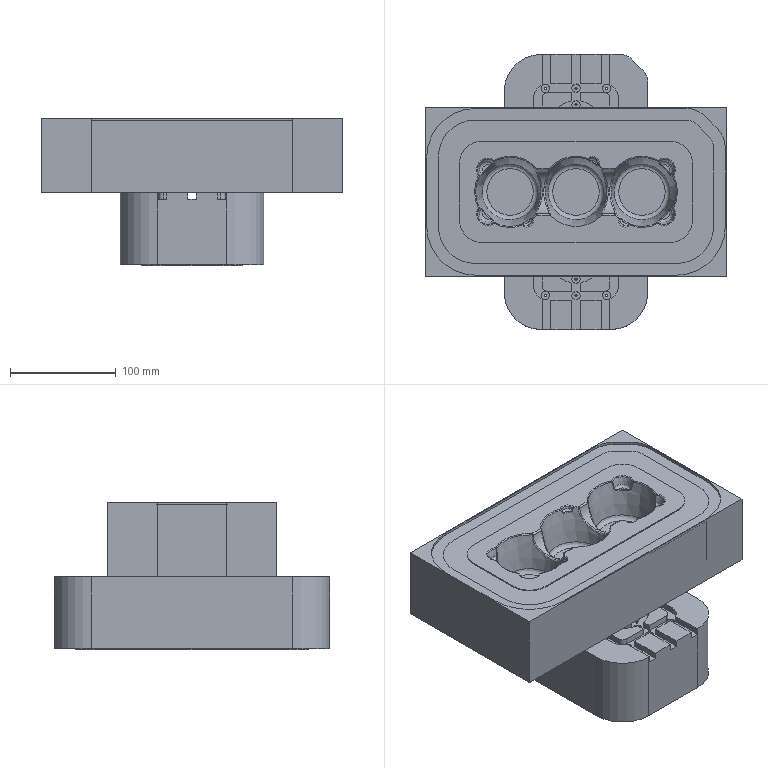NC program | NX | posted with a generic post | part box 284.317 x 260.317 x 139.5 mm
Lines 198484 to 199234 of 226982:
(B6 , TOOL : D10)
N396948 M6
N396950 G53
N396952 G17 G0 G90 X62.725 Y73.878 S7000 M3 M8
N396954 G43 Z220.5 H0
N396956 Z70.
N396958 G94 G1 X100.887 Z68. F4000.
N396960 X103.946
N396962 G2 X118.795 Y67.727 R21.
N396964 G1 X130.008 Y56.514
N396966 G2 X136.159 Y41.664 R21.
N396968 G1 Y-32.878
N396970 G2 X95.159 Y-73.878 R41.
N396972 G1 X-95.159
N396974 G2 X-136.159 Y-32.878 R41.
N396976 G1 Y32.878
N396978 G2 X-95.159 Y73.878 R41.
N396980 G1 X100.887
N396982 Y66.878
N396984 X103.946
N396986 G2 X113.845 Y62.777 R14.
N396988 G1 X125.058 Y51.564
N396990 G2 X129.159 Y41.664 R14.
N396992 G1 Y-32.878
N396994 G2 X95.159 Y-66.878 R34.
N396996 G1 X-95.159
N396998 G2 X-129.159 Y-32.878 R34.
N397000 G1 Y32.878
N397002 G2 X-95.159 Y66.878 R34.
N397004 G1 X100.887
N397006 Y59.878
N397008 X103.946
N397010 G2 X108.895 Y57.827 R7.
N397012 G1 X120.108 Y46.614
N397014 G2 X122.159 Y41.664 R7.
N397016 G1 Y-32.878
N397018 G2 X100.008 Y-59.439 R27.
N397020 G1 X98.751 Y-52.552
N397022 G3 X114.834 Y-36.469 R27.372
N397024 G2 X98.751 Y-52.552 R20.
N397026 G1 X93.926 Y-53.864
N397028 G2 X89.187 Y-54.278 R27.372
N397030 G1 X-89.187
N397032 G2 X-93.926 Y-53.864 R27.372
N397034 X-94.324 Y-54.878 R5.
N397036 G1 X94.324
N397038 G2 X93.926 Y-53.864 R5.
N397040 G1 X98.751 Y-52.552
N397042 X100.008 Y-59.439
N397044 G2 X95.159 Y-59.878 R27.
N397046 G1 X-95.159
N397048 G2 X-121.72 Y-37.726 R27.
N397050 G1 X-114.834 Y-36.469
N397052 G3 X-98.751 Y-52.552 R27.372
N397054 G2 X-114.834 Y-36.469 R20.
N397056 G1 X-121.72 Y-37.726
N397058 G2 X-122.159 Y-32.878 R27.
N397060 G1 Y32.878
N397062 G2 X-100.008 Y59.439 R27.
N397064 G1 X-98.751 Y52.552
N397066 G3 X-114.834 Y36.469 R27.372
N397068 G1 X-117.159 Y32.043
N397070 Y-32.043
N397072 G2 X-116.145 Y-31.644 R5.
N397074 X-116.559 Y-26.906 R27.372
N397076 G1 Y26.906
N397078 G2 X-116.145 Y31.644 R27.372
N397080 X-117.159 Y32.043 R5.
N397082 G1 X-114.834 Y36.469
N397084 G2 X-98.751 Y52.552 R20.
N397086 G1 X-93.926 Y53.864
N397088 G2 X-89.187 Y54.278 R27.372
N397090 G1 X89.187
N397092 G2 X92.96 Y54.016 R27.372
N397094 X93.246 Y54.878 R5.
N397096 G1 X-94.324
N397098 G2 X-93.926 Y53.864 R5.
N397100 G1 X-98.751 Y52.552
N397102 X-100.008 Y59.439
N397104 G2 X-95.159 Y59.878 R27.
N397106 G1 X100.887
N397108 Y52.878
N397110 X103.946
N397112 X115.159 Y41.664
N397114 Y35.547
N397116 X116.297 Y30.679
N397118 G2 X116.559 Y26.906 R27.372
N397120 G1 Y-26.906
N397122 G2 X116.145 Y-31.644 R27.372
N397124 X117.159 Y-32.043 R5.
N397126 G1 Y30.965
N397128 G2 X116.297 Y30.679 R5.
N397130 G1 X115.159 Y35.547
N397132 G3 X97.829 Y52.878 R27.372
N397134 G1 X97.387 Y51.549
N397136 G2 X115.159 Y26.906 R25.972
N397138 G1 Y-26.906
N397140 G2 X89.187 Y-52.878 R25.972
N397142 G1 X-89.187
N397144 G2 X-115.159 Y-26.906 R25.972
N397146 G1 Y26.906
N397148 G2 X-89.187 Y52.878 R25.972
N397150 G1 X89.187
N397152 G2 X97.387 Y51.549 R25.972
N397154 G1 X97.829 Y52.878
N397156 X100.887
N397158 G3 X102.887 Y54.878 R2.
N397160 G1 Z69.
N397162 G0 Z220.5
(B7 , TOOL : D10)
N397164 X53.127 Y72.878
N397166 Z69.
N397168 G1 X105.041 Z68.955
N397170 X107.727 Y72.547 Z68.952
N397172 X110.343 Y71.858 Z68.95
N397174 X112.843 Y70.823 Z68.948
N397176 X115.18 Y69.46 Z68.945
N397178 X117.313 Y67.795 Z68.943
N397180 X130.076 Y55.032 Z68.927
N397182 X131.741 Y52.899 Z68.925
N397184 X133.104 Y50.562 Z68.922
N397186 X134.14 Y48.062 Z68.92
N397188 X134.829 Y45.446 Z68.918
N397190 X135.159 Y42.76 Z68.915
N397192 Y-34.427 Z68.848
N397194 X134.766 Y-38.677 Z68.844
N397196 X133.924 Y-42.861 Z68.841
N397198 X132.641 Y-46.931 Z68.837
N397200 X130.931 Y-50.842 Z68.833
N397202 X128.815 Y-54.548 Z68.829
N397204 X126.317 Y-58.009 Z68.826
N397206 X123.464 Y-61.183 Z68.822
N397208 X120.29 Y-64.036 Z68.818
N397210 X116.83 Y-66.534 Z68.814
N397212 X113.123 Y-68.65 Z68.811
N397214 X109.212 Y-70.359 Z68.807
N397216 X105.142 Y-71.643 Z68.803
N397218 X100.958 Y-72.485 Z68.8
N397220 X96.708 Y-72.878 Z68.796
N397222 X-96.708 Z68.627
N397224 X-100.958 Y-72.485 Z68.623
N397226 X-105.142 Y-71.643 Z68.62
N397228 X-109.212 Y-70.359 Z68.616
N397230 X-113.123 Y-68.65 Z68.612
N397232 X-116.83 Y-66.534 Z68.608
N397234 X-120.29 Y-64.036 Z68.605
N397236 X-123.464 Y-61.183 Z68.601
N397238 X-126.317 Y-58.009 Z68.597
N397240 X-128.815 Y-54.548 Z68.594
N397242 X-130.931 Y-50.842 Z68.59
N397244 X-132.641 Y-46.931 Z68.586
N397246 X-133.924 Y-42.861 Z68.582
N397248 X-134.766 Y-38.677 Z68.579
N397250 X-135.159 Y-34.427 Z68.575
N397252 Y34.427 Z68.515
N397254 X-134.766 Y38.677 Z68.511
N397256 X-133.924 Y42.861 Z68.507
N397258 X-132.641 Y46.931 Z68.504
N397260 X-130.931 Y50.842 Z68.5
N397262 X-128.815 Y54.548 Z68.496
N397264 X-126.317 Y58.009 Z68.492
N397266 X-123.464 Y61.183 Z68.489
N397268 X-120.29 Y64.036 Z68.485
N397270 X-116.83 Y66.534 Z68.481
N397272 X-113.123 Y68.65 Z68.478
N397274 X-109.212 Y70.359 Z68.474
N397276 X-105.142 Y71.643 Z68.47
N397278 X-100.958 Y72.485 Z68.466
N397280 X-96.708 Y72.878 Z68.463
N397282 X105.041 Z68.287
N397284 X107.727 Y72.547 Z68.284
N397286 X110.343 Y71.858 Z68.282
N397288 X112.843 Y70.823 Z68.28
N397290 X115.18 Y69.46 Z68.277
N397292 X117.313 Y67.795 Z68.275
N397294 X130.076 Y55.032 Z68.259
N397296 X131.741 Y52.899 Z68.257
N397298 X133.104 Y50.562 Z68.254
N397300 X134.14 Y48.062 Z68.252
N397302 X134.829 Y45.446 Z68.25
N397304 X135.159 Y42.76 Z68.247
N397306 Y-34.427 Z68.18
N397308 X134.766 Y-38.677 Z68.176
N397310 X133.924 Y-42.861 Z68.172
N397312 X132.641 Y-46.931 Z68.169
N397314 X130.931 Y-50.842 Z68.165
N397316 X128.815 Y-54.548 Z68.161
N397318 X126.317 Y-58.009 Z68.158
N397320 X123.464 Y-61.183 Z68.154
N397322 X120.29 Y-64.036 Z68.15
N397324 X116.83 Y-66.534 Z68.146
N397326 X113.123 Y-68.65 Z68.143
N397328 X109.212 Y-70.359 Z68.139
N397330 X105.142 Y-71.643 Z68.135
N397332 X100.958 Y-72.485 Z68.131
N397334 X96.708 Y-72.878 Z68.128
N397336 X-96.708 Z67.959
N397338 X-100.958 Y-72.485 Z67.955
N397340 X-105.142 Y-71.643 Z67.952
N397342 X-109.212 Y-70.359 Z67.948
N397344 X-113.123 Y-68.65 Z67.944
N397346 X-116.83 Y-66.534 Z67.94
N397348 X-120.29 Y-64.036 Z67.937
N397350 X-123.464 Y-61.183 Z67.933
N397352 X-126.317 Y-58.009 Z67.929
N397354 X-128.815 Y-54.548 Z67.925
N397356 X-130.931 Y-50.842 Z67.922
N397358 X-132.641 Y-46.931 Z67.918
N397360 X-133.924 Y-42.861 Z67.914
N397362 X-134.766 Y-38.677 Z67.911
N397364 X-135.159 Y-34.427 Z67.907
N397366 Y34.427 Z67.847
N397368 X-134.766 Y38.677 Z67.843
N397370 X-133.924 Y42.861 Z67.839
N397372 X-132.641 Y46.931 Z67.836
N397374 X-130.931 Y50.842 Z67.832
N397376 X-128.815 Y54.548 Z67.828
N397378 X-126.317 Y58.009 Z67.824
N397380 X-123.464 Y61.183 Z67.821
N397382 X-120.29 Y64.036 Z67.817
N397384 X-116.83 Y66.534 Z67.813
N397386 X-113.123 Y68.65 Z67.809
N397388 X-109.212 Y70.359 Z67.806
N397390 X-105.142 Y71.643 Z67.802
N397392 X-100.958 Y72.485 Z67.798
N397394 X-96.708 Y72.878 Z67.795
N397396 X105.041 Z67.619
N397398 X107.727 Y72.547 Z67.616
N397400 X110.343 Y71.858 Z67.614
N397402 X112.843 Y70.823 Z67.611
N397404 X115.18 Y69.46 Z67.609
N397406 X117.313 Y67.795 Z67.607
N397408 X130.076 Y55.032 Z67.591
N397410 X131.741 Y52.899 Z67.589
N397412 X133.104 Y50.562 Z67.586
N397414 X134.14 Y48.062 Z67.584
N397416 X134.829 Y45.446 Z67.582
N397418 X135.159 Y42.76 Z67.579
N397420 Y-34.427 Z67.512
N397422 X134.766 Y-38.677 Z67.508
N397424 X133.924 Y-42.861 Z67.504
N397426 X132.641 Y-46.931 Z67.501
N397428 X130.931 Y-50.842 Z67.497
N397430 X128.815 Y-54.548 Z67.493
N397432 X126.317 Y-58.009 Z67.489
N397434 X123.464 Y-61.183 Z67.486
N397436 X120.29 Y-64.036 Z67.482
N397438 X116.83 Y-66.534 Z67.478
N397440 X113.123 Y-68.65 Z67.475
N397442 X109.212 Y-70.359 Z67.471
N397444 X105.142 Y-71.643 Z67.467
N397446 X100.958 Y-72.485 Z67.463
N397448 X96.708 Y-72.878 Z67.46
N397450 X-96.708 Z67.291
N397452 X-100.958 Y-72.485 Z67.287
N397454 X-105.142 Y-71.643 Z67.283
N397456 X-109.212 Y-70.359 Z67.28
N397458 X-113.123 Y-68.65 Z67.276
N397460 X-116.83 Y-66.534 Z67.272
N397462 X-120.29 Y-64.036 Z67.269
N397464 X-123.464 Y-61.183 Z67.265
N397466 X-126.317 Y-58.009 Z67.261
N397468 X-128.815 Y-54.548 Z67.257
N397470 X-130.931 Y-50.842 Z67.254
N397472 X-132.641 Y-46.931 Z67.25
N397474 X-133.924 Y-42.861 Z67.246
N397476 X-134.766 Y-38.677 Z67.242
N397478 X-135.159 Y-34.427 Z67.239
N397480 Y34.427 Z67.179
N397482 X-134.766 Y38.677 Z67.175
N397484 X-133.924 Y42.861 Z67.171
N397486 X-132.641 Y46.931 Z67.167
N397488 X-130.931 Y50.842 Z67.164
N397490 X-128.815 Y54.548 Z67.16
N397492 X-126.317 Y58.009 Z67.156
N397494 X-123.464 Y61.183 Z67.153
N397496 X-120.29 Y64.036 Z67.149
N397498 X-116.83 Y66.534 Z67.145
N397500 X-113.123 Y68.65 Z67.141
N397502 X-109.212 Y70.359 Z67.138
N397504 X-105.142 Y71.643 Z67.134
N397506 X-100.958 Y72.485 Z67.13
N397508 X-96.708 Y72.878 Z67.127
N397510 X105.041 Z66.95
N397512 X107.727 Y72.547 Z66.948
N397514 X110.343 Y71.858 Z66.946
N397516 X112.843 Y70.823 Z66.943
N397518 X115.18 Y69.46 Z66.941
N397520 X117.313 Y67.795 Z66.939
N397522 X130.076 Y55.032 Z66.923
N397524 X131.741 Y52.899 Z66.921
N397526 X133.104 Y50.562 Z66.918
N397528 X134.14 Y48.062 Z66.916
N397530 X134.829 Y45.446 Z66.913
N397532 X135.159 Y42.76 Z66.911
N397534 Y-34.427 Z66.844
N397536 X134.766 Y-38.677 Z66.84
N397538 X133.924 Y-42.861 Z66.836
N397540 X132.641 Y-46.931 Z66.833
N397542 X130.931 Y-50.842 Z66.829
N397544 X128.815 Y-54.548 Z66.825
N397546 X126.317 Y-58.009 Z66.821
N397548 X123.464 Y-61.183 Z66.818
N397550 X120.29 Y-64.036 Z66.814
N397552 X116.83 Y-66.534 Z66.81
N397554 X113.123 Y-68.65 Z66.806
N397556 X109.212 Y-70.359 Z66.803
N397558 X105.142 Y-71.643 Z66.799
N397560 X100.958 Y-72.485 Z66.795
N397562 X96.708 Y-72.878 Z66.792
N397564 X-96.708 Z66.623
N397566 X-100.958 Y-72.485 Z66.619
N397568 X-105.142 Y-71.643 Z66.615
N397570 X-109.212 Y-70.359 Z66.612
N397572 X-113.123 Y-68.65 Z66.608
N397574 X-116.83 Y-66.534 Z66.604
N397576 X-120.29 Y-64.036 Z66.6
N397578 X-123.464 Y-61.183 Z66.597
N397580 X-126.317 Y-58.009 Z66.593
N397582 X-128.815 Y-54.548 Z66.589
N397584 X-130.931 Y-50.842 Z66.586
N397586 X-132.641 Y-46.931 Z66.582
N397588 X-133.924 Y-42.861 Z66.578
N397590 X-134.766 Y-38.677 Z66.574
N397592 X-135.159 Y-34.427 Z66.571
N397594 Y34.427 Z66.511
N397596 X-134.766 Y38.677 Z66.507
N397598 X-133.924 Y42.861 Z66.503
N397600 X-132.641 Y46.931 Z66.499
N397602 X-130.931 Y50.842 Z66.496
N397604 X-128.815 Y54.548 Z66.492
N397606 X-126.317 Y58.009 Z66.488
N397608 X-123.464 Y61.183 Z66.484
N397610 X-120.29 Y64.036 Z66.481
N397612 X-116.83 Y66.534 Z66.477
N397614 X-113.123 Y68.65 Z66.473
N397616 X-109.212 Y70.359 Z66.47
N397618 X-105.142 Y71.643 Z66.466
N397620 X-100.958 Y72.485 Z66.462
N397622 X-96.708 Y72.878 Z66.458
N397624 X105.041 Z66.282
N397626 X107.727 Y72.547 Z66.28
N397628 X110.343 Y71.858 Z66.278
N397630 X112.843 Y70.823 Z66.275
N397632 X115.18 Y69.46 Z66.273
N397634 X117.313 Y67.795 Z66.271
N397636 X130.076 Y55.032 Z66.255
N397638 X131.741 Y52.899 Z66.252
N397640 X133.104 Y50.562 Z66.25
N397642 X134.14 Y48.062 Z66.248
N397644 X134.829 Y45.446 Z66.245
N397646 X135.159 Y42.76 Z66.243
N397648 Y-34.427 Z66.176
N397650 X134.766 Y-38.677 Z66.172
N397652 X133.924 Y-42.861 Z66.168
N397654 X132.641 Y-46.931 Z66.164
N397656 X130.931 Y-50.842 Z66.161
N397658 X128.815 Y-54.548 Z66.157
N397660 X126.317 Y-58.009 Z66.153
N397662 X123.464 Y-61.183 Z66.15
N397664 X120.29 Y-64.036 Z66.146
N397666 X116.83 Y-66.534 Z66.142
N397668 X113.123 Y-68.65 Z66.138
N397670 X109.212 Y-70.359 Z66.135
N397672 X105.142 Y-71.643 Z66.131
N397674 X100.958 Y-72.485 Z66.127
N397676 X96.708 Y-72.878 Z66.124
N397678 X-96.708 Z65.955
N397680 X-100.958 Y-72.485 Z65.951
N397682 X-105.142 Y-71.643 Z65.947
N397684 X-109.212 Y-70.359 Z65.944
N397686 X-113.123 Y-68.65 Z65.94
N397688 X-116.83 Y-66.534 Z65.936
N397690 X-120.29 Y-64.036 Z65.932
N397692 X-123.464 Y-61.183 Z65.929
N397694 X-126.317 Y-58.009 Z65.925
N397696 X-128.815 Y-54.548 Z65.921
N397698 X-130.931 Y-50.842 Z65.917
N397700 X-132.641 Y-46.931 Z65.914
N397702 X-133.924 Y-42.861 Z65.91
N397704 X-134.766 Y-38.677 Z65.906
N397706 X-135.159 Y-34.427 Z65.903
N397708 Y34.427 Z65.842
N397710 X-134.766 Y38.677 Z65.839
N397712 X-133.924 Y42.861 Z65.835
N397714 X-132.641 Y46.931 Z65.831
N397716 X-130.931 Y50.842 Z65.828
N397718 X-128.815 Y54.548 Z65.824
N397720 X-126.317 Y58.009 Z65.82
N397722 X-123.464 Y61.183 Z65.816
N397724 X-120.29 Y64.036 Z65.813
N397726 X-116.83 Y66.534 Z65.809
N397728 X-113.123 Y68.65 Z65.805
N397730 X-109.212 Y70.359 Z65.802
N397732 X-105.142 Y71.643 Z65.798
N397734 X-100.958 Y72.485 Z65.794
N397736 X-96.708 Y72.878 Z65.79
N397738 X105.041 Z65.614
N397740 X107.727 Y72.547 Z65.612
N397742 X110.343 Y71.858 Z65.61
N397744 X112.843 Y70.823 Z65.607
N397746 X115.18 Y69.46 Z65.605
N397748 X117.313 Y67.795 Z65.602
N397750 X130.076 Y55.032 Z65.587
N397752 X131.741 Y52.899 Z65.584
N397754 X133.104 Y50.562 Z65.582
N397756 X134.14 Y48.062 Z65.58
N397758 X134.829 Y45.446 Z65.577
N397760 X135.159 Y42.76 Z65.575
N397762 Y-34.427 Z65.508
N397764 X134.766 Y-38.677 Z65.504
N397766 X133.924 Y-42.861 Z65.5
N397768 X132.641 Y-46.931 Z65.496
N397770 X130.931 Y-50.842 Z65.493
N397772 X128.815 Y-54.548 Z65.489
N397774 X126.317 Y-58.009 Z65.485
N397776 X123.464 Y-61.183 Z65.481
N397778 X120.29 Y-64.036 Z65.478
N397780 X116.83 Y-66.534 Z65.474
N397782 X113.123 Y-68.65 Z65.47
N397784 X109.212 Y-70.359 Z65.467
N397786 X105.142 Y-71.643 Z65.463
N397788 X100.958 Y-72.485 Z65.459
N397790 X96.708 Y-72.878 Z65.455
N397792 X-96.708 Z65.287
N397794 X-100.958 Y-72.485 Z65.283
N397796 X-105.142 Y-71.643 Z65.279
N397798 X-109.212 Y-70.359 Z65.275
N397800 X-113.123 Y-68.65 Z65.272
N397802 X-116.83 Y-66.534 Z65.268
N397804 X-120.29 Y-64.036 Z65.264
N397806 X-123.464 Y-61.183 Z65.261
N397808 X-126.317 Y-58.009 Z65.257
N397810 X-128.815 Y-54.548 Z65.253
N397812 X-130.931 Y-50.842 Z65.249
N397814 X-132.641 Y-46.931 Z65.246
N397816 X-133.924 Y-42.861 Z65.242
N397818 X-134.766 Y-38.677 Z65.238
N397820 X-135.159 Y-34.427 Z65.234
N397822 Y34.427 Z65.174
N397824 X-134.766 Y38.677 Z65.171
N397826 X-133.924 Y42.861 Z65.167
N397828 X-132.641 Y46.931 Z65.163
N397830 X-130.931 Y50.842 Z65.16
N397832 X-128.815 Y54.548 Z65.156
N397834 X-126.317 Y58.009 Z65.152
N397836 X-123.464 Y61.183 Z65.148
N397838 X-120.29 Y64.036 Z65.145
N397840 X-116.83 Y66.534 Z65.141
N397842 X-113.123 Y68.65 Z65.137
N397844 X-109.212 Y70.359 Z65.133
N397846 X-105.142 Y71.643 Z65.13
N397848 X-100.958 Y72.485 Z65.126
N397850 X-96.708 Y72.878 Z65.122
N397852 X105.041 Z64.946
N397854 X107.727 Y72.547 Z64.944
N397856 X110.343 Y71.858 Z64.941
N397858 X112.843 Y70.823 Z64.939
N397860 X115.18 Y69.46 Z64.937
N397862 X117.313 Y67.795 Z64.934
N397864 X130.076 Y55.032 Z64.919
N397866 X131.741 Y52.899 Z64.916
N397868 X133.104 Y50.562 Z64.914
N397870 X134.14 Y48.062 Z64.912
N397872 X134.829 Y45.446 Z64.909
N397874 X135.159 Y42.76 Z64.907
N397876 Y-34.427 Z64.839
N397878 X134.766 Y-38.677 Z64.836
N397880 X133.924 Y-42.861 Z64.832
N397882 X132.641 Y-46.931 Z64.828
N397884 X130.931 Y-50.842 Z64.825
N397886 X128.815 Y-54.548 Z64.821
N397888 X126.317 Y-58.009 Z64.817
N397890 X123.464 Y-61.183 Z64.813
N397892 X120.29 Y-64.036 Z64.81
N397894 X116.83 Y-66.534 Z64.806
N397896 X113.123 Y-68.65 Z64.802
N397898 X109.212 Y-70.359 Z64.799
N397900 X105.142 Y-71.643 Z64.795
N397902 X100.958 Y-72.485 Z64.791
N397904 X96.708 Y-72.878 Z64.787
N397906 X-96.708 Z64.619
N397908 X-100.958 Y-72.485 Z64.615
N397910 X-105.142 Y-71.643 Z64.611
N397912 X-109.212 Y-70.359 Z64.607
N397914 X-113.123 Y-68.65 Z64.604
N397916 X-116.83 Y-66.534 Z64.6
N397918 X-120.29 Y-64.036 Z64.596
N397920 X-123.464 Y-61.183 Z64.592
N397922 X-126.317 Y-58.009 Z64.589
N397924 X-128.815 Y-54.548 Z64.585
N397926 X-130.931 Y-50.842 Z64.581
N397928 X-132.641 Y-46.931 Z64.578
N397930 X-133.924 Y-42.861 Z64.574
N397932 X-134.766 Y-38.677 Z64.57
N397934 X-135.159 Y-34.427 Z64.566
N397936 Y34.427 Z64.506
N397938 X-134.766 Y38.677 Z64.503
N397940 X-133.924 Y42.861 Z64.499
N397942 X-132.641 Y46.931 Z64.495
N397944 X-130.931 Y50.842 Z64.491
N397946 X-128.815 Y54.548 Z64.488
N397948 X-126.317 Y58.009 Z64.484
N397950 X-123.464 Y61.183 Z64.48
N397952 X-120.29 Y64.036 Z64.477
N397954 X-116.83 Y66.534 Z64.473
N397956 X-113.123 Y68.65 Z64.469
N397958 X-109.212 Y70.359 Z64.465
N397960 X-105.142 Y71.643 Z64.462
N397962 X-100.958 Y72.485 Z64.458
N397964 X-96.708 Y72.878 Z64.454
N397966 X105.041 Z64.278
N397968 X107.727 Y72.547 Z64.276
N397970 X110.343 Y71.858 Z64.273
N397972 X112.843 Y70.823 Z64.271
N397974 X115.18 Y69.46 Z64.269
N397976 X117.313 Y67.795 Z64.266
N397978 X130.076 Y55.032 Z64.251
N397980 X131.741 Y52.899 Z64.248
N397982 X133.104 Y50.562 Z64.246
N397984 X134.14 Y48.062 Z64.243
N397986 X134.829 Y45.446 Z64.241
N397988 X135.159 Y42.76 Z64.239
N397990 Y-34.427 Z64.171
N397992 X134.766 Y-38.677 Z64.168
N397994 X133.924 Y-42.861 Z64.164
N397996 X132.641 Y-46.931 Z64.16
N397998 X130.931 Y-50.842 Z64.156
N398000 X128.815 Y-54.548 Z64.153
N398002 X126.317 Y-58.009 Z64.149
N398004 X123.464 Y-61.183 Z64.145
N398006 X120.29 Y-64.036 Z64.142
N398008 X116.83 Y-66.534 Z64.138
N398010 X113.123 Y-68.65 Z64.134
N398012 X109.212 Y-70.359 Z64.13
N398014 X105.142 Y-71.643 Z64.127
N398016 X100.958 Y-72.485 Z64.123
N398018 X96.708 Y-72.878 Z64.119
N398020 X-96.708 Z63.95
N398022 X-100.958 Y-72.485 Z63.947
N398024 X-105.142 Y-71.643 Z63.943
N398026 X-109.212 Y-70.359 Z63.939
N398028 X-113.123 Y-68.65 Z63.936
N398030 X-116.83 Y-66.534 Z63.932
N398032 X-120.29 Y-64.036 Z63.928
N398034 X-123.464 Y-61.183 Z63.924
N398036 X-126.317 Y-58.009 Z63.921
N398038 X-128.815 Y-54.548 Z63.917
N398040 X-130.931 Y-50.842 Z63.913
N398042 X-132.641 Y-46.931 Z63.909
N398044 X-133.924 Y-42.861 Z63.906
N398046 X-134.766 Y-38.677 Z63.902
N398048 X-135.159 Y-34.427 Z63.898
N398050 Y34.427 Z63.838
N398052 X-134.766 Y38.677 Z63.835
N398054 X-133.924 Y42.861 Z63.831
N398056 X-132.641 Y46.931 Z63.827
N398058 X-130.931 Y50.842 Z63.823
N398060 X-128.815 Y54.548 Z63.82
N398062 X-126.317 Y58.009 Z63.816
N398064 X-123.464 Y61.183 Z63.812
N398066 X-120.29 Y64.036 Z63.808
N398068 X-116.83 Y66.534 Z63.805
N398070 X-113.123 Y68.65 Z63.801
N398072 X-109.212 Y70.359 Z63.797
N398074 X-105.142 Y71.643 Z63.794
N398076 X-100.958 Y72.485 Z63.79
N398078 X-96.708 Y72.878 Z63.786
N398080 X105.041 Z63.61
N398082 X107.727 Y72.547 Z63.608
N398084 X110.343 Y71.858 Z63.605
N398086 X112.843 Y70.823 Z63.603
N398088 X115.18 Y69.46 Z63.601
N398090 X117.313 Y67.795 Z63.598
N398092 X130.076 Y55.032 Z63.582
N398094 X131.741 Y52.899 Z63.58
N398096 X133.104 Y50.562 Z63.578
N398098 X134.14 Y48.062 Z63.575
N398100 X134.829 Y45.446 Z63.573
N398102 X135.159 Y42.76 Z63.571
N398104 Y-34.427 Z63.503
N398106 X134.766 Y-38.677 Z63.5
N398108 X133.924 Y-42.861 Z63.496
N398110 X132.641 Y-46.931 Z63.492
N398112 X130.931 Y-50.842 Z63.488
N398114 X128.815 Y-54.548 Z63.485
N398116 X126.317 Y-58.009 Z63.481
N398118 X123.464 Y-61.183 Z63.477
N398120 X120.29 Y-64.036 Z63.474
N398122 X116.83 Y-66.534 Z63.47
N398124 X113.123 Y-68.65 Z63.466
N398126 X109.212 Y-70.359 Z63.462
N398128 X105.142 Y-71.643 Z63.459
N398130 X100.958 Y-72.485 Z63.455
N398132 X96.708 Y-72.878 Z63.451
N398134 X-96.708 Z63.282
N398136 X-100.958 Y-72.485 Z63.279
N398138 X-105.142 Y-71.643 Z63.275
N398140 X-109.212 Y-70.359 Z63.271
N398142 X-113.123 Y-68.65 Z63.267
N398144 X-116.83 Y-66.534 Z63.264
N398146 X-120.29 Y-64.036 Z63.26
N398148 X-123.464 Y-61.183 Z63.256
N398150 X-126.317 Y-58.009 Z63.253
N398152 X-128.815 Y-54.548 Z63.249
N398154 X-130.931 Y-50.842 Z63.245
N398156 X-132.641 Y-46.931 Z63.241
N398158 X-133.924 Y-42.861 Z63.238
N398160 X-134.766 Y-38.677 Z63.234
N398162 X-135.159 Y-34.427 Z63.23
N398164 Y34.427 Z63.17
N398166 X-134.766 Y38.677 Z63.166
N398168 X-133.924 Y42.861 Z63.163
N398170 X-132.641 Y46.931 Z63.159
N398172 X-130.931 Y50.842 Z63.155
N398174 X-128.815 Y54.548 Z63.152
N398176 X-126.317 Y58.009 Z63.148
N398178 X-123.464 Y61.183 Z63.144
N398180 X-120.29 Y64.036 Z63.14
N398182 X-116.83 Y66.534 Z63.137
N398184 X-113.123 Y68.65 Z63.133
N398186 X-109.212 Y70.359 Z63.129
N398188 X-105.142 Y71.643 Z63.125
N398190 X-100.958 Y72.485 Z63.122
N398192 X-96.708 Y72.878 Z63.118
N398194 X105.041 Z62.942
N398196 X107.727 Y72.547 Z62.94
N398198 X110.343 Y71.858 Z62.937
N398200 X112.843 Y70.823 Z62.935
N398202 X115.18 Y69.46 Z62.933
N398204 X117.313 Y67.795 Z62.93
N398206 X130.076 Y55.032 Z62.914
N398208 X131.741 Y52.899 Z62.912
N398210 X133.104 Y50.562 Z62.91
N398212 X134.14 Y48.062 Z62.907
N398214 X134.829 Y45.446 Z62.905
N398216 X135.159 Y42.76 Z62.903
N398218 Y-34.427 Z62.835
N398220 X134.766 Y-38.677 Z62.832
N398222 X133.924 Y-42.861 Z62.828
N398224 X132.641 Y-46.931 Z62.824
N398226 X130.931 Y-50.842 Z62.82
N398228 X128.815 Y-54.548 Z62.817
N398230 X126.317 Y-58.009 Z62.813
N398232 X123.464 Y-61.183 Z62.809
N398234 X120.29 Y-64.036 Z62.805
N398236 X116.83 Y-66.534 Z62.802
N398238 X113.123 Y-68.65 Z62.798
N398240 X109.212 Y-70.359 Z62.794
N398242 X105.142 Y-71.643 Z62.791
N398244 X100.958 Y-72.485 Z62.787
N398246 X96.708 Y-72.878 Z62.783
N398248 X-96.708 Z62.614
N398250 X-100.958 Y-72.485 Z62.611
N398252 X-105.142 Y-71.643 Z62.607
N398254 X-109.212 Y-70.359 Z62.603
N398256 X-113.123 Y-68.65 Z62.599
N398258 X-116.83 Y-66.534 Z62.596
N398260 X-120.29 Y-64.036 Z62.592
N398262 X-123.464 Y-61.183 Z62.588
N398264 X-126.317 Y-58.009 Z62.585
N398266 X-128.815 Y-54.548 Z62.581
N398268 X-130.931 Y-50.842 Z62.577
N398270 X-132.641 Y-46.931 Z62.573
N398272 X-133.924 Y-42.861 Z62.57
N398274 X-134.766 Y-38.677 Z62.566
N398276 X-135.159 Y-34.427 Z62.562
N398278 Y34.427 Z62.502
N398280 X-134.766 Y38.677 Z62.498
N398282 X-133.924 Y42.861 Z62.495
N398284 X-132.641 Y46.931 Z62.491
N398286 X-130.931 Y50.842 Z62.487
N398288 X-128.815 Y54.548 Z62.483
N398290 X-126.317 Y58.009 Z62.48
N398292 X-123.464 Y61.183 Z62.476
N398294 X-120.29 Y64.036 Z62.472
N398296 X-116.83 Y66.534 Z62.469
N398298 X-113.123 Y68.65 Z62.465
N398300 X-109.212 Y70.359 Z62.461
N398302 X-105.142 Y71.643 Z62.457
N398304 X-100.958 Y72.485 Z62.454
N398306 X-96.708 Y72.878 Z62.45
N398308 X105.041 Z62.274
N398310 X107.727 Y72.547 Z62.272
N398312 X110.343 Y71.858 Z62.269
N398314 X112.843 Y70.823 Z62.267
N398316 X115.18 Y69.46 Z62.264
N398318 X117.313 Y67.795 Z62.262
N398320 X130.076 Y55.032 Z62.246
N398322 X131.741 Y52.899 Z62.244
N398324 X133.104 Y50.562 Z62.242
N398326 X134.14 Y48.062 Z62.239
N398328 X134.829 Y45.446 Z62.237
N398330 X135.159 Y42.76 Z62.235
N398332 Y-34.427 Z62.167
N398334 X134.766 Y-38.677 Z62.163
N398336 X133.924 Y-42.861 Z62.16
N398338 X132.641 Y-46.931 Z62.156
N398340 X130.931 Y-50.842 Z62.152
N398342 X128.815 Y-54.548 Z62.149
N398344 X126.317 Y-58.009 Z62.145
N398346 X123.464 Y-61.183 Z62.141
N398348 X120.29 Y-64.036 Z62.137
N398350 X116.83 Y-66.534 Z62.134
N398352 X113.123 Y-68.65 Z62.13
N398354 X109.212 Y-70.359 Z62.126
N398356 X105.142 Y-71.643 Z62.122
N398358 X100.958 Y-72.485 Z62.119
N398360 X96.708 Y-72.878 Z62.115
N398362 X-96.708 Z61.946
N398364 X-100.958 Y-72.485 Z61.942
N398366 X-105.142 Y-71.643 Z61.939
N398368 X-109.212 Y-70.359 Z61.935
N398370 X-113.123 Y-68.65 Z61.931
N398372 X-116.83 Y-66.534 Z61.928
N398374 X-120.29 Y-64.036 Z61.924
N398376 X-123.464 Y-61.183 Z61.92
N398378 X-126.317 Y-58.009 Z61.916
N398380 X-128.815 Y-54.548 Z61.913
N398382 X-130.931 Y-50.842 Z61.909
N398384 X-132.641 Y-46.931 Z61.905
N398386 X-133.924 Y-42.861 Z61.902
N398388 X-134.766 Y-38.677 Z61.898
N398390 X-135.159 Y-34.427 Z61.894
N398392 Y34.427 Z61.834
N398394 X-134.766 Y38.677 Z61.83
N398396 X-133.924 Y42.861 Z61.827
N398398 X-132.641 Y46.931 Z61.823
N398400 X-130.931 Y50.842 Z61.819
N398402 X-128.815 Y54.548 Z61.815
N398404 X-126.317 Y58.009 Z61.812
N398406 X-123.464 Y61.183 Z61.808
N398408 X-120.29 Y64.036 Z61.804
N398410 X-116.83 Y66.534 Z61.8
N398412 X-113.123 Y68.65 Z61.797
N398414 X-109.212 Y70.359 Z61.793
N398416 X-105.142 Y71.643 Z61.789
N398418 X-100.958 Y72.485 Z61.786
N398420 X-96.708 Y72.878 Z61.782
N398422 X105.041 Z61.606
N398424 X107.727 Y72.547 Z61.603
N398426 X110.343 Y71.858 Z61.601
N398428 X112.843 Y70.823 Z61.599
N398430 X115.18 Y69.46 Z61.596
N398432 X117.313 Y67.795 Z61.594
N398434 X130.076 Y55.032 Z61.578
N398436 X131.741 Y52.899 Z61.576